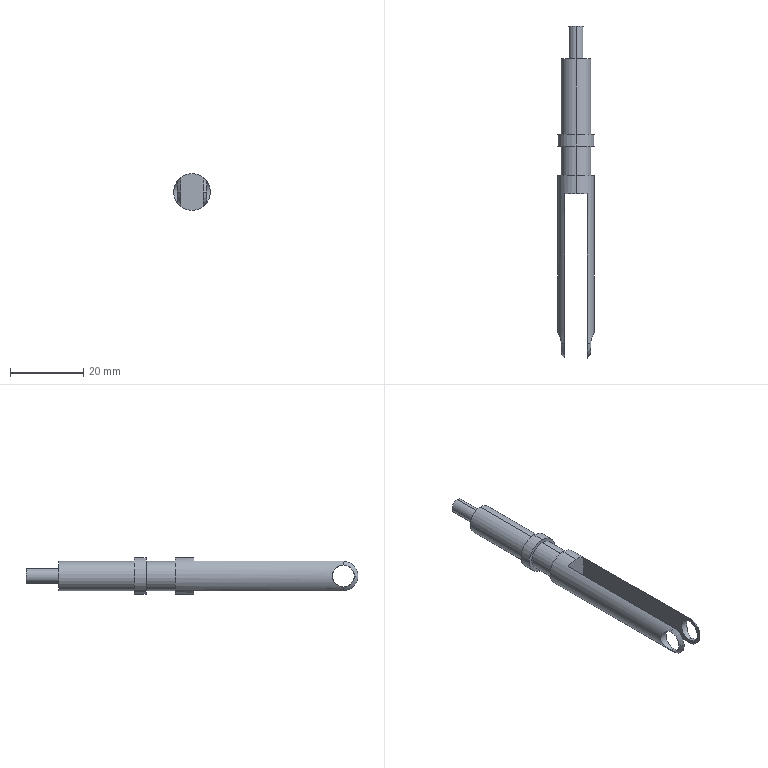Part | SolidWorks | features ICE 2, Revolution 1 | 1 solid | 26 faces | box 10 x 90.414 x 10 mm | volume 3064 mm3 | cylinder 14 | plane 8 | sphere 4 | commonest cylinder face diameters 6 x4 8 x4 10 x4 4 x2
STEP:
#1=CARTESIAN_POINT('',(-29.291,-51.374,3.));
#2=VERTEX_POINT('',#1);
#3=CARTESIAN_POINT('',(-29.291,-51.374,-3.));
#4=VERTEX_POINT('',#3);
#5=CARTESIAN_POINT('',(-29.291,-51.374,0.));
#6=DIRECTION('',(1.,0.,0.));
#7=DIRECTION('',(0.,0.,-1.));
#8=AXIS2_PLACEMENT_3D('',#5,#6,#7);
#9=CIRCLE('',#8,3.);
#10=EDGE_CURVE('',#2,#4,#9,.T.);
#11=ORIENTED_EDGE('',*,*,#10,.F.);
#12=CARTESIAN_POINT('',(-28.291,-51.374,3.));
#13=VERTEX_POINT('',#12);
#14=CARTESIAN_POINT('',(-54.291,-51.374,3.));
#15=DIRECTION('',(1.,0.,0.));
#16=VECTOR('',#15,1000.);
#17=LINE('',#14,#16);
#18=EDGE_CURVE('',#2,#13,#17,.T.);
#19=ORIENTED_EDGE('',*,*,#18,.T.);
#20=CARTESIAN_POINT('',(-28.291,-54.374,0.));
#21=VERTEX_POINT('',#20);
#22=CARTESIAN_POINT('',(-28.291,-51.374,0.));
#23=DIRECTION('',(1.,0.,0.));
#24=DIRECTION('',(0.,0.,1.));
#25=AXIS2_PLACEMENT_3D('',#22,#23,#24);
#26=CIRCLE('',#25,3.);
#27=EDGE_CURVE('',#13,#21,#26,.T.);
#28=ORIENTED_EDGE('',*,*,#27,.T.);
#29=CARTESIAN_POINT('',(-28.291,-51.374,-3.));
#30=VERTEX_POINT('',#29);
#31=CARTESIAN_POINT('',(-28.291,-51.374,0.));
#32=DIRECTION('',(1.,0.,0.));
#33=DIRECTION('',(0.,0.,1.));
#34=AXIS2_PLACEMENT_3D('',#31,#32,#33);
#35=CIRCLE('',#34,3.);
#36=EDGE_CURVE('',#21,#30,#35,.T.);
#37=ORIENTED_EDGE('',*,*,#36,.T.);
#38=CARTESIAN_POINT('',(-54.291,-51.374,-3.));
#39=DIRECTION('',(1.,0.,0.));
#40=VECTOR('',#39,1000.);
#41=LINE('',#38,#40);
#42=EDGE_CURVE('',#4,#30,#41,.T.);
#43=ORIENTED_EDGE('',*,*,#42,.F.);
#44=EDGE_LOOP('',(#11,#19,#28,#37,#43));
#45=FACE_OUTER_BOUND('',#44,.T.);
#46=CARTESIAN_POINT('',(-54.291,-51.374,0.));
#47=DIRECTION('',(1.,0.,0.));
#48=DIRECTION('',(0.,0.,-1.));
#49=AXIS2_PLACEMENT_3D('',#46,#47,#48);
#50=CYLINDRICAL_SURFACE('',#49,3.);
#51=ADVANCED_FACE('',(#45),#50,.F.);
#52=CARTESIAN_POINT('',(-36.291,-54.374,0.));
#53=VERTEX_POINT('',#52);
#54=CARTESIAN_POINT('',(-36.291,-51.374,3.));
#55=VERTEX_POINT('',#54);
#56=CARTESIAN_POINT('',(-36.291,-51.374,0.));
#57=DIRECTION('',(-1.,0.,0.));
#58=DIRECTION('',(0.,0.,-1.));
#59=AXIS2_PLACEMENT_3D('',#56,#57,#58);
#60=CIRCLE('',#59,3.);
#61=EDGE_CURVE('',#53,#55,#60,.T.);
#62=ORIENTED_EDGE('',*,*,#61,.T.);
#63=CARTESIAN_POINT('',(-35.291,-51.374,3.));
#64=VERTEX_POINT('',#63);
#65=CARTESIAN_POINT('',(-54.291,-51.374,3.));
#66=DIRECTION('',(1.,0.,0.));
#67=VECTOR('',#66,1000.);
#68=LINE('',#65,#67);
#69=EDGE_CURVE('',#55,#64,#68,.T.);
#70=ORIENTED_EDGE('',*,*,#69,.T.);
#71=CARTESIAN_POINT('',(-35.291,-51.374,-3.));
#72=VERTEX_POINT('',#71);
#73=CARTESIAN_POINT('',(-35.291,-51.374,0.));
#74=DIRECTION('',(-1.,0.,0.));
#75=DIRECTION('',(0.,0.,1.));
#76=AXIS2_PLACEMENT_3D('',#73,#74,#75);
#77=CIRCLE('',#76,3.);
#78=EDGE_CURVE('',#72,#64,#77,.T.);
#79=ORIENTED_EDGE('',*,*,#78,.F.);
#80=CARTESIAN_POINT('',(-36.291,-51.374,-3.));
#81=VERTEX_POINT('',#80);
#82=CARTESIAN_POINT('',(-54.291,-51.374,-3.));
#83=DIRECTION('',(1.,0.,0.));
#84=VECTOR('',#83,1000.);
#85=LINE('',#82,#84);
#86=EDGE_CURVE('',#81,#72,#85,.T.);
#87=ORIENTED_EDGE('',*,*,#86,.F.);
#88=CARTESIAN_POINT('',(-36.291,-51.374,0.));
#89=DIRECTION('',(-1.,0.,0.));
#90=DIRECTION('',(0.,0.,-1.));
#91=AXIS2_PLACEMENT_3D('',#88,#89,#90);
#92=CIRCLE('',#91,3.);
#93=EDGE_CURVE('',#81,#53,#92,.T.);
#94=ORIENTED_EDGE('',*,*,#93,.T.);
#95=EDGE_LOOP('',(#62,#70,#79,#87,#94));
#96=FACE_OUTER_BOUND('',#95,.T.);
#97=CARTESIAN_POINT('',(-54.291,-51.374,0.));
#98=DIRECTION('',(1.,0.,0.));
#99=DIRECTION('',(0.,0.,-1.));
#100=AXIS2_PLACEMENT_3D('',#97,#98,#99);
#101=CYLINDRICAL_SURFACE('',#100,3.);
#102=ADVANCED_FACE('',(#96),#101,.F.);
#103=ORIENTED_EDGE('',*,*,#61,.F.);
#104=CARTESIAN_POINT('',(-35.291,-55.374,0.));
#105=VERTEX_POINT('',#104);
#106=CARTESIAN_POINT('',(-32.291,-51.374,0.));
#107=DIRECTION('',(0.,0.,1.));
#108=DIRECTION('',(1.,0.,0.));
#109=AXIS2_PLACEMENT_3D('',#106,#107,#108);
#110=CIRCLE('',#109,5.);
#111=EDGE_CURVE('',#53,#105,#110,.T.);
#112=ORIENTED_EDGE('',*,*,#111,.T.);
#113=CARTESIAN_POINT('',(-35.291,-51.374,4.));
#114=VERTEX_POINT('',#113);
#115=CARTESIAN_POINT('',(-35.291,-51.374,0.));
#116=DIRECTION('',(1.,0.,0.));
#117=DIRECTION('',(0.,0.,1.));
#118=AXIS2_PLACEMENT_3D('',#115,#116,#117);
#119=CIRCLE('',#118,4.);
#120=EDGE_CURVE('',#114,#105,#119,.T.);
#121=ORIENTED_EDGE('',*,*,#120,.F.);
#122=CARTESIAN_POINT('',(-32.291,-51.374,0.));
#123=DIRECTION('',(0.,-1.,0.));
#124=DIRECTION('',(0.,0.,-1.));
#125=AXIS2_PLACEMENT_3D('',#122,#123,#124);
#126=CIRCLE('',#125,5.);
#127=EDGE_CURVE('',#114,#55,#126,.T.);
#128=ORIENTED_EDGE('',*,*,#127,.T.);
#129=EDGE_LOOP('',(#103,#112,#121,#128));
#130=FACE_OUTER_BOUND('',#129,.T.);
#131=CARTESIAN_POINT('',(-32.291,-51.374,0.));
#132=DIRECTION('',(0.,0.,-1.));
#133=DIRECTION('',(-1.,0.,0.));
#134=AXIS2_PLACEMENT_3D('',#131,#132,#133);
#135=SPHERICAL_SURFACE('',#134,5.);
#136=ADVANCED_FACE('',(#130),#135,.T.);
#137=CARTESIAN_POINT('',(-32.291,35.041,-2.));
#138=VERTEX_POINT('',#137);
#139=CARTESIAN_POINT('',(-32.291,35.041,2.));
#140=VERTEX_POINT('',#139);
#141=CARTESIAN_POINT('',(-32.291,35.041,0.));
#142=DIRECTION('',(0.,-1.,0.));
#143=DIRECTION('',(0.,0.,-1.));
#144=AXIS2_PLACEMENT_3D('',#141,#142,#143);
#145=CIRCLE('',#144,2.);
#146=EDGE_CURVE('',#138,#140,#145,.T.);
#147=ORIENTED_EDGE('',*,*,#146,.T.);
#148=CARTESIAN_POINT('',(-32.291,26.124,2.));
#149=VERTEX_POINT('',#148);
#150=CARTESIAN_POINT('',(-32.291,35.041,2.));
#151=DIRECTION('',(0.,-1.,0.));
#152=VECTOR('',#151,1000.);
#153=LINE('',#150,#152);
#154=EDGE_CURVE('',#140,#149,#153,.T.);
#155=ORIENTED_EDGE('',*,*,#154,.T.);
#156=CARTESIAN_POINT('',(-32.291,26.124,-2.));
#157=VERTEX_POINT('',#156);
#158=CARTESIAN_POINT('',(-32.291,26.124,0.));
#159=DIRECTION('',(0.,-1.,0.));
#160=DIRECTION('',(0.,0.,-1.));
#161=AXIS2_PLACEMENT_3D('',#158,#159,#160);
#162=CIRCLE('',#161,2.);
#163=EDGE_CURVE('',#157,#149,#162,.T.);
#164=ORIENTED_EDGE('',*,*,#163,.F.);
#165=CARTESIAN_POINT('',(-32.291,35.041,-2.));
#166=DIRECTION('',(0.,-1.,0.));
#167=VECTOR('',#166,1000.);
#168=LINE('',#165,#167);
#169=EDGE_CURVE('',#138,#157,#168,.T.);
#170=ORIENTED_EDGE('',*,*,#169,.F.);
#171=EDGE_LOOP('',(#147,#155,#164,#170));
#172=FACE_OUTER_BOUND('',#171,.T.);
#173=CARTESIAN_POINT('',(-32.291,35.041,0.));
#174=DIRECTION('',(0.,-1.,0.));
#175=DIRECTION('',(0.,0.,-1.));
#176=AXIS2_PLACEMENT_3D('',#173,#174,#175);
#177=CYLINDRICAL_SURFACE('',#176,2.);
#178=ADVANCED_FACE('',(#172),#177,.T.);
#179=CARTESIAN_POINT('',(-32.291,26.124,-4.));
#180=VERTEX_POINT('',#179);
#181=CARTESIAN_POINT('',(-32.291,26.124,4.));
#182=VERTEX_POINT('',#181);
#183=CARTESIAN_POINT('',(-32.291,26.124,0.));
#184=DIRECTION('',(0.,-1.,0.));
#185=DIRECTION('',(0.,0.,-1.));
#186=AXIS2_PLACEMENT_3D('',#183,#184,#185);
#187=CIRCLE('',#186,4.);
#188=EDGE_CURVE('',#180,#182,#187,.T.);
#189=ORIENTED_EDGE('',*,*,#188,.T.);
#190=CARTESIAN_POINT('',(-32.291,5.494,4.));
#191=VERTEX_POINT('',#190);
#192=CARTESIAN_POINT('',(-32.291,35.041,4.));
#193=DIRECTION('',(0.,-1.,0.));
#194=VECTOR('',#193,1000.);
#195=LINE('',#192,#194);
#196=EDGE_CURVE('',#182,#191,#195,.T.);
#197=ORIENTED_EDGE('',*,*,#196,.T.);
#198=CARTESIAN_POINT('',(-32.291,5.494,-4.));
#199=VERTEX_POINT('',#198);
#200=CARTESIAN_POINT('',(-32.291,5.494,0.));
#201=DIRECTION('',(0.,-1.,0.));
#202=DIRECTION('',(0.,0.,-1.));
#203=AXIS2_PLACEMENT_3D('',#200,#201,#202);
#204=CIRCLE('',#203,4.);
#205=EDGE_CURVE('',#199,#191,#204,.T.);
#206=ORIENTED_EDGE('',*,*,#205,.F.);
#207=CARTESIAN_POINT('',(-32.291,35.041,-4.));
#208=DIRECTION('',(0.,-1.,0.));
#209=VECTOR('',#208,1000.);
#210=LINE('',#207,#209);
#211=EDGE_CURVE('',#180,#199,#210,.T.);
#212=ORIENTED_EDGE('',*,*,#211,.F.);
#213=EDGE_LOOP('',(#189,#197,#206,#212));
#214=FACE_OUTER_BOUND('',#213,.T.);
#215=CARTESIAN_POINT('',(-32.291,35.041,0.));
#216=DIRECTION('',(0.,-1.,0.));
#217=DIRECTION('',(0.,0.,-1.));
#218=AXIS2_PLACEMENT_3D('',#215,#216,#217);
#219=CYLINDRICAL_SURFACE('',#218,4.);
#220=ADVANCED_FACE('',(#214),#219,.T.);
#221=CARTESIAN_POINT('',(-32.291,5.494,-5.));
#222=VERTEX_POINT('',#221);
#223=CARTESIAN_POINT('',(-32.291,5.494,5.));
#224=VERTEX_POINT('',#223);
#225=CARTESIAN_POINT('',(-32.291,5.494,0.));
#226=DIRECTION('',(0.,-1.,0.));
#227=DIRECTION('',(0.,0.,-1.));
#228=AXIS2_PLACEMENT_3D('',#225,#226,#227);
#229=CIRCLE('',#228,5.);
#230=EDGE_CURVE('',#222,#224,#229,.T.);
#231=ORIENTED_EDGE('',*,*,#230,.T.);
#232=CARTESIAN_POINT('',(-32.291,2.336,5.));
#233=VERTEX_POINT('',#232);
#234=CARTESIAN_POINT('',(-32.291,35.041,5.));
#235=DIRECTION('',(0.,-1.,0.));
#236=VECTOR('',#235,1000.);
#237=LINE('',#234,#236);
#238=EDGE_CURVE('',#224,#233,#237,.T.);
#239=ORIENTED_EDGE('',*,*,#238,.T.);
#240=CARTESIAN_POINT('',(-32.291,2.336,-5.));
#241=VERTEX_POINT('',#240);
#242=CARTESIAN_POINT('',(-32.291,2.336,0.));
#243=DIRECTION('',(0.,-1.,0.));
#244=DIRECTION('',(0.,0.,-1.));
#245=AXIS2_PLACEMENT_3D('',#242,#243,#244);
#246=CIRCLE('',#245,5.);
#247=EDGE_CURVE('',#241,#233,#246,.T.);
#248=ORIENTED_EDGE('',*,*,#247,.F.);
#249=CARTESIAN_POINT('',(-32.291,35.041,-5.));
#250=DIRECTION('',(0.,-1.,0.));
#251=VECTOR('',#250,1000.);
#252=LINE('',#249,#251);
#253=EDGE_CURVE('',#222,#241,#252,.T.);
#254=ORIENTED_EDGE('',*,*,#253,.F.);
#255=EDGE_LOOP('',(#231,#239,#248,#254));
#256=FACE_OUTER_BOUND('',#255,.T.);
#257=CARTESIAN_POINT('',(-32.291,35.041,0.));
#258=DIRECTION('',(0.,-1.,0.));
#259=DIRECTION('',(0.,0.,-1.));
#260=AXIS2_PLACEMENT_3D('',#257,#258,#259);
#261=CYLINDRICAL_SURFACE('',#260,5.);
#262=ADVANCED_FACE('',(#256),#261,.T.);
#263=CARTESIAN_POINT('',(-32.291,2.336,-4.));
#264=VERTEX_POINT('',#263);
#265=CARTESIAN_POINT('',(-32.291,2.336,4.));
#266=VERTEX_POINT('',#265);
#267=CARTESIAN_POINT('',(-32.291,2.336,0.));
#268=DIRECTION('',(0.,-1.,0.));
#269=DIRECTION('',(0.,0.,-1.));
#270=AXIS2_PLACEMENT_3D('',#267,#268,#269);
#271=CIRCLE('',#270,4.);
#272=EDGE_CURVE('',#264,#266,#271,.T.);
#273=ORIENTED_EDGE('',*,*,#272,.T.);
#274=CARTESIAN_POINT('',(-32.291,-5.664,4.));
#275=VERTEX_POINT('',#274);
#276=CARTESIAN_POINT('',(-32.291,35.041,4.));
#277=DIRECTION('',(0.,-1.,0.));
#278=VECTOR('',#277,1000.);
#279=LINE('',#276,#278);
#280=EDGE_CURVE('',#266,#275,#279,.T.);
#281=ORIENTED_EDGE('',*,*,#280,.T.);
#282=CARTESIAN_POINT('',(-32.291,-5.664,-4.));
#283=VERTEX_POINT('',#282);
#284=CARTESIAN_POINT('',(-32.291,-5.664,0.));
#285=DIRECTION('',(0.,-1.,0.));
#286=DIRECTION('',(0.,0.,-1.));
#287=AXIS2_PLACEMENT_3D('',#284,#285,#286);
#288=CIRCLE('',#287,4.);
#289=EDGE_CURVE('',#283,#275,#288,.T.);
#290=ORIENTED_EDGE('',*,*,#289,.F.);
#291=CARTESIAN_POINT('',(-32.291,35.041,-4.));
#292=DIRECTION('',(0.,-1.,0.));
#293=VECTOR('',#292,1000.);
#294=LINE('',#291,#293);
#295=EDGE_CURVE('',#264,#283,#294,.T.);
#296=ORIENTED_EDGE('',*,*,#295,.F.);
#297=EDGE_LOOP('',(#273,#281,#290,#296));
#298=FACE_OUTER_BOUND('',#297,.T.);
#299=CARTESIAN_POINT('',(-32.291,35.041,0.));
#300=DIRECTION('',(0.,-1.,0.));
#301=DIRECTION('',(0.,0.,-1.));
#302=AXIS2_PLACEMENT_3D('',#299,#300,#301);
#303=CYLINDRICAL_SURFACE('',#302,4.);
#304=ADVANCED_FACE('',(#298),#303,.T.);
#305=CARTESIAN_POINT('',(-32.291,-5.664,-5.));
#306=VERTEX_POINT('',#305);
#307=CARTESIAN_POINT('',(-32.291,-5.664,5.));
#308=VERTEX_POINT('',#307);
#309=CARTESIAN_POINT('',(-32.291,-5.664,0.));
#310=DIRECTION('',(0.,-1.,0.));
#311=DIRECTION('',(0.,0.,-1.));
#312=AXIS2_PLACEMENT_3D('',#309,#310,#311);
#313=CIRCLE('',#312,5.);
#314=EDGE_CURVE('',#306,#308,#313,.T.);
#315=ORIENTED_EDGE('',*,*,#314,.T.);
#316=CARTESIAN_POINT('',(-32.291,-10.664,5.));
#317=VERTEX_POINT('',#316);
#318=CARTESIAN_POINT('',(-32.291,35.041,5.));
#319=DIRECTION('',(0.,-1.,0.));
#320=VECTOR('',#319,1000.);
#321=LINE('',#318,#320);
#322=EDGE_CURVE('',#308,#317,#321,.T.);
#323=ORIENTED_EDGE('',*,*,#322,.T.);
#324=CARTESIAN_POINT('',(-29.291,-10.664,4.));
#325=VERTEX_POINT('',#324);
#326=CARTESIAN_POINT('',(-32.291,-10.664,0.));
#327=DIRECTION('',(0.,1.,0.));
#328=DIRECTION('',(0.,0.,-1.));
#329=AXIS2_PLACEMENT_3D('',#326,#327,#328);
#330=CIRCLE('',#329,5.);
#331=EDGE_CURVE('',#317,#325,#330,.T.);
#332=ORIENTED_EDGE('',*,*,#331,.T.);
#333=CARTESIAN_POINT('',(-29.291,-51.374,4.));
#334=VERTEX_POINT('',#333);
#335=CARTESIAN_POINT('',(-29.291,35.041,4.));
#336=DIRECTION('',(0.,1.,0.));
#337=VECTOR('',#336,1000.);
#338=LINE('',#335,#337);
#339=EDGE_CURVE('',#334,#325,#338,.T.);
#340=ORIENTED_EDGE('',*,*,#339,.F.);
#341=CARTESIAN_POINT('',(-32.291,-51.374,0.));
#342=DIRECTION('',(0.,-1.,0.));
#343=DIRECTION('',(0.,0.,-1.));
#344=AXIS2_PLACEMENT_3D('',#341,#342,#343);
#345=CIRCLE('',#344,5.);
#346=EDGE_CURVE('',#13,#334,#345,.T.);
#347=ORIENTED_EDGE('',*,*,#346,.F.);
#348=CARTESIAN_POINT('',(-28.291,-51.374,-3.));
#349=CARTESIAN_POINT('',(-28.291,-51.17,-3.));
#350=CARTESIAN_POINT('',(-28.275,-50.971,-2.979));
#351=CARTESIAN_POINT('',(-28.218,-50.581,-2.9));
#352=CARTESIAN_POINT('',(-28.175,-50.389,-2.841));
#353=CARTESIAN_POINT('',(-28.025,-49.85,-2.614));
#354=CARTESIAN_POINT('',(-27.892,-49.527,-2.395));
#355=CARTESIAN_POINT('',(-27.702,-49.121,-1.991));
#356=CARTESIAN_POINT('',(-27.639,-48.997,-1.841));
#357=CARTESIAN_POINT('',(-27.525,-48.78,-1.521));
#358=CARTESIAN_POINT('',(-27.474,-48.688,-1.351));
#359=CARTESIAN_POINT('',(-27.387,-48.535,-0.9904));
#360=CARTESIAN_POINT('',(-27.351,-48.474,-0.7969));
#361=CARTESIAN_POINT('',(-27.304,-48.395,-0.4064));
#362=CARTESIAN_POINT('',(-27.291,-48.374,-0.2077));
#363=CARTESIAN_POINT('',(-27.291,-48.373,0.197));
#364=CARTESIAN_POINT('',(-27.303,-48.394,0.3998));
#365=CARTESIAN_POINT('',(-27.35,-48.473,0.7912));
#366=CARTESIAN_POINT('',(-27.385,-48.533,0.9841));
#367=CARTESIAN_POINT('',(-27.516,-48.763,1.529));
#368=CARTESIAN_POINT('',(-27.638,-48.985,1.855));
#369=CARTESIAN_POINT('',(-27.828,-49.391,2.259));
#370=CARTESIAN_POINT('',(-27.893,-49.54,2.382));
#371=CARTESIAN_POINT('',(-28.017,-49.86,2.597));
#372=CARTESIAN_POINT('',(-28.074,-50.028,2.689));
#373=CARTESIAN_POINT('',(-28.175,-50.386,2.84));
#374=CARTESIAN_POINT('',(-28.217,-50.578,2.9));
#375=CARTESIAN_POINT('',(-28.275,-50.97,2.979));
#376=CARTESIAN_POINT('',(-28.291,-51.169,3.));
#377=CARTESIAN_POINT('',(-28.291,-51.374,3.));
#378=B_SPLINE_CURVE_WITH_KNOTS('',3,(#348,#349,#350,#351,#352,#353,#354,#355,#356,#357,#358,#359,#360,#361,#362,#363,#364,#365,#366,#367,#368,#369,#370,#371,#372,#373,#374,#375,#376,#377),.UNSPECIFIED.,.F.,.F.,(4,2,2,2,2,2,2,2,2,2,2,2,2,2,4),(0.,0.0006013,0.001203,0.002405,0.003007,0.003608,0.004209,0.00481,0.005412,0.006013,0.007216,0.007817,0.008418,0.00902,0.009621),.UNSPECIFIED.);
#379=EDGE_CURVE('',#30,#13,#378,.T.);
#380=ORIENTED_EDGE('',*,*,#379,.F.);
#381=CARTESIAN_POINT('',(-29.291,-51.374,-4.));
#382=VERTEX_POINT('',#381);
#383=CARTESIAN_POINT('',(-32.291,-51.374,0.));
#384=DIRECTION('',(0.,-1.,0.));
#385=DIRECTION('',(0.,0.,-1.));
#386=AXIS2_PLACEMENT_3D('',#383,#384,#385);
#387=CIRCLE('',#386,5.);
#388=EDGE_CURVE('',#382,#30,#387,.T.);
#389=ORIENTED_EDGE('',*,*,#388,.F.);
#390=CARTESIAN_POINT('',(-29.291,-10.664,-4.));
#391=VERTEX_POINT('',#390);
#392=CARTESIAN_POINT('',(-29.291,35.041,-4.));
#393=DIRECTION('',(0.,-1.,0.));
#394=VECTOR('',#393,1000.);
#395=LINE('',#392,#394);
#396=EDGE_CURVE('',#391,#382,#395,.T.);
#397=ORIENTED_EDGE('',*,*,#396,.F.);
#398=CARTESIAN_POINT('',(-32.291,-10.664,-5.));
#399=VERTEX_POINT('',#398);
#400=CARTESIAN_POINT('',(-32.291,-10.664,0.));
#401=DIRECTION('',(0.,1.,0.));
#402=DIRECTION('',(0.,0.,-1.));
#403=AXIS2_PLACEMENT_3D('',#400,#401,#402);
#404=CIRCLE('',#403,5.);
#405=EDGE_CURVE('',#391,#399,#404,.T.);
#406=ORIENTED_EDGE('',*,*,#405,.T.);
#407=CARTESIAN_POINT('',(-32.291,35.041,-5.));
#408=DIRECTION('',(0.,-1.,0.));
#409=VECTOR('',#408,1000.);
#410=LINE('',#407,#409);
#411=EDGE_CURVE('',#306,#399,#410,.T.);
#412=ORIENTED_EDGE('',*,*,#411,.F.);
#413=EDGE_LOOP('',(#315,#323,#332,#340,#347,#380,#389,#397,#406,#412));
#414=FACE_OUTER_BOUND('',#413,.T.);
#415=CARTESIAN_POINT('',(-32.291,35.041,0.));
#416=DIRECTION('',(0.,-1.,0.));
#417=DIRECTION('',(0.,0.,-1.));
#418=AXIS2_PLACEMENT_3D('',#415,#416,#417);
#419=CYLINDRICAL_SURFACE('',#418,5.);
#420=ADVANCED_FACE('',(#414),#419,.T.);
#421=ORIENTED_EDGE('',*,*,#36,.F.);
#422=CARTESIAN_POINT('',(-29.291,-55.374,0.));
#423=VERTEX_POINT('',#422);
#424=CARTESIAN_POINT('',(-32.291,-51.374,0.));
#425=DIRECTION('',(0.,0.,-1.));
#426=DIRECTION('',(-1.,0.,0.));
#427=AXIS2_PLACEMENT_3D('',#424,#425,#426);
#428=CIRCLE('',#427,5.);
#429=EDGE_CURVE('',#21,#423,#428,.T.);
#430=ORIENTED_EDGE('',*,*,#429,.T.);
#431=CARTESIAN_POINT('',(-29.291,-51.374,0.));
#432=DIRECTION('',(-1.,0.,0.));
#433=DIRECTION('',(0.,0.,-1.));
#434=AXIS2_PLACEMENT_3D('',#431,#432,#433);
#435=CIRCLE('',#434,4.);
#436=EDGE_CURVE('',#382,#423,#435,.T.);
#437=ORIENTED_EDGE('',*,*,#436,.F.);
#438=ORIENTED_EDGE('',*,*,#388,.T.);
#439=EDGE_LOOP('',(#421,#430,#437,#438));
#440=FACE_OUTER_BOUND('',#439,.T.);
#441=CARTESIAN_POINT('',(-32.291,-51.374,0.));
#442=DIRECTION('',(0.,0.,-1.));
#443=DIRECTION('',(-1.,0.,0.));
#444=AXIS2_PLACEMENT_3D('',#441,#442,#443);
#445=SPHERICAL_SURFACE('',#444,5.);
#446=ADVANCED_FACE('',(#440),#445,.T.);
#447=ORIENTED_EDGE('',*,*,#429,.F.);
#448=ORIENTED_EDGE('',*,*,#27,.F.);
#449=ORIENTED_EDGE('',*,*,#346,.T.);
#450=CARTESIAN_POINT('',(-29.291,-51.374,0.));
#451=DIRECTION('',(-1.,0.,0.));
#452=DIRECTION('',(0.,0.,-1.));
#453=AXIS2_PLACEMENT_3D('',#450,#451,#452);
#454=CIRCLE('',#453,4.);
#455=EDGE_CURVE('',#423,#334,#454,.T.);
#456=ORIENTED_EDGE('',*,*,#455,.F.);
#457=EDGE_LOOP('',(#447,#448,#449,#456));
#458=FACE_OUTER_BOUND('',#457,.T.);
#459=CARTESIAN_POINT('',(-32.291,-51.374,0.));
#460=DIRECTION('',(0.,0.,-1.));
#461=DIRECTION('',(-1.,0.,0.));
#462=AXIS2_PLACEMENT_3D('',#459,#460,#461);
#463=SPHERICAL_SURFACE('',#462,5.);
#464=ADVANCED_FACE('',(#458),#463,.T.);
#465=ORIENTED_EDGE('',*,*,#322,.F.);
#466=CARTESIAN_POINT('',(-32.291,-5.664,0.));
#467=DIRECTION('',(0.,-1.,0.));
#468=DIRECTION('',(0.,0.,-1.));
#469=AXIS2_PLACEMENT_3D('',#466,#467,#468);
#470=CIRCLE('',#469,5.);
#471=EDGE_CURVE('',#308,#306,#470,.T.);
#472=ORIENTED_EDGE('',*,*,#471,.T.);
#473=ORIENTED_EDGE('',*,*,#411,.T.);
#474=CARTESIAN_POINT('',(-35.291,-10.664,-4.));
#475=VERTEX_POINT('',#474);
#476=CARTESIAN_POINT('',(-32.291,-10.664,0.));
#477=DIRECTION('',(0.,1.,0.));
#478=DIRECTION('',(0.,0.,-1.));
#479=AXIS2_PLACEMENT_3D('',#476,#477,#478);
#480=CIRCLE('',#479,5.);
#481=EDGE_CURVE('',#399,#475,#480,.T.);
#482=ORIENTED_EDGE('',*,*,#481,.T.);
#483=CARTESIAN_POINT('',(-35.291,-51.374,-4.));
#484=VERTEX_POINT('',#483);
#485=CARTESIAN_POINT('',(-35.291,35.041,-4.));
#486=DIRECTION('',(0.,1.,0.));
#487=VECTOR('',#486,1000.);
#488=LINE('',#485,#487);
#489=EDGE_CURVE('',#484,#475,#488,.T.);
#490=ORIENTED_EDGE('',*,*,#489,.F.);
#491=CARTESIAN_POINT('',(-32.291,-51.374,0.));
#492=DIRECTION('',(0.,-1.,0.));
#493=DIRECTION('',(0.,0.,-1.));
#494=AXIS2_PLACEMENT_3D('',#491,#492,#493);
#495=CIRCLE('',#494,5.);
#496=EDGE_CURVE('',#81,#484,#495,.T.);
#497=ORIENTED_EDGE('',*,*,#496,.F.);
#498=CARTESIAN_POINT('',(-36.291,-51.374,3.));
#499=CARTESIAN_POINT('',(-36.291,-51.17,3.));
#500=CARTESIAN_POINT('',(-36.307,-50.971,2.979));
#501=CARTESIAN_POINT('',(-36.364,-50.581,2.9));
#502=CARTESIAN_POINT('',(-36.407,-50.389,2.841));
#503=CARTESIAN_POINT('',(-36.558,-49.85,2.614));
#504=CARTESIAN_POINT('',(-36.69,-49.527,2.395));
#505=CARTESIAN_POINT('',(-36.88,-49.121,1.991));
#506=CARTESIAN_POINT('',(-36.943,-48.997,1.841));
#507=CARTESIAN_POINT('',(-37.057,-48.78,1.521));
#508=CARTESIAN_POINT('',(-37.109,-48.688,1.351));
#509=CARTESIAN_POINT('',(-37.196,-48.535,0.9904));
#510=CARTESIAN_POINT('',(-37.231,-48.474,0.7969));
#511=CARTESIAN_POINT('',(-37.278,-48.395,0.4064));
#512=CARTESIAN_POINT('',(-37.291,-48.374,0.2077));
#513=CARTESIAN_POINT('',(-37.291,-48.373,-0.197));
#514=CARTESIAN_POINT('',(-37.279,-48.394,-0.3998));
#515=CARTESIAN_POINT('',(-37.232,-48.473,-0.7912));
#516=CARTESIAN_POINT('',(-37.197,-48.533,-0.9841));
#517=CARTESIAN_POINT('',(-37.066,-48.763,-1.529));
#518=CARTESIAN_POINT('',(-36.944,-48.985,-1.855));
#519=CARTESIAN_POINT('',(-36.754,-49.391,-2.259));
#520=CARTESIAN_POINT('',(-36.689,-49.54,-2.382));
#521=CARTESIAN_POINT('',(-36.566,-49.86,-2.597));
#522=CARTESIAN_POINT('',(-36.508,-50.028,-2.689));
#523=CARTESIAN_POINT('',(-36.408,-50.386,-2.84));
#524=CARTESIAN_POINT('',(-36.365,-50.578,-2.9));
#525=CARTESIAN_POINT('',(-36.307,-50.97,-2.979));
#526=CARTESIAN_POINT('',(-36.291,-51.169,-3.));
#527=CARTESIAN_POINT('',(-36.291,-51.374,-3.));
#528=B_SPLINE_CURVE_WITH_KNOTS('',3,(#498,#499,#500,#501,#502,#503,#504,#505,#506,#507,#508,#509,#510,#511,#512,#513,#514,#515,#516,#517,#518,#519,#520,#521,#522,#523,#524,#525,#526,#527),.UNSPECIFIED.,.F.,.F.,(4,2,2,2,2,2,2,2,2,2,2,2,2,2,4),(0.,0.0006013,0.001203,0.002405,0.003007,0.003608,0.004209,0.00481,0.005412,0.006013,0.007216,0.007817,0.008418,0.00902,0.009621),.UNSPECIFIED.);
#529=EDGE_CURVE('',#55,#81,#528,.T.);
#530=ORIENTED_EDGE('',*,*,#529,.F.);
#531=ORIENTED_EDGE('',*,*,#127,.F.);
#532=CARTESIAN_POINT('',(-35.291,-10.664,4.));
#533=VERTEX_POINT('',#532);
#534=CARTESIAN_POINT('',(-35.291,35.041,4.));
#535=DIRECTION('',(0.,-1.,0.));
#536=VECTOR('',#535,1000.);
#537=LINE('',#534,#536);
#538=EDGE_CURVE('',#533,#114,#537,.T.);
#539=ORIENTED_EDGE('',*,*,#538,.F.);
#540=CARTESIAN_POINT('',(-32.291,-10.664,0.));
#541=DIRECTION('',(0.,1.,0.));
#542=DIRECTION('',(0.,0.,-1.));
#543=AXIS2_PLACEMENT_3D('',#540,#541,#542);
#544=CIRCLE('',#543,5.);
#545=EDGE_CURVE('',#533,#317,#544,.T.);
#546=ORIENTED_EDGE('',*,*,#545,.T.);
#547=EDGE_LOOP('',(#465,#472,#473,#482,#490,#497,#530,#531,#539,#546));
#548=FACE_OUTER_BOUND('',#547,.T.);
#549=CARTESIAN_POINT('',(-32.291,35.041,0.));
#550=DIRECTION('',(0.,-1.,0.));
#551=DIRECTION('',(0.,0.,-1.));
#552=AXIS2_PLACEMENT_3D('',#549,#550,#551);
#553=CYLINDRICAL_SURFACE('',#552,5.);
#554=ADVANCED_FACE('',(#548),#553,.T.);
#555=ORIENTED_EDGE('',*,*,#289,.T.);
#556=CARTESIAN_POINT('',(-32.291,-5.664,0.));
#557=DIRECTION('',(0.,-1.,0.));
#558=DIRECTION('',(0.,0.,-1.));
#559=AXIS2_PLACEMENT_3D('',#556,#557,#558);
#560=CIRCLE('',#559,4.);
#561=EDGE_CURVE('',#275,#283,#560,.T.);
#562=ORIENTED_EDGE('',*,*,#561,.T.);
#563=EDGE_LOOP('',(#555,#562));
#564=FACE_BOUND('',#563,.T.);
#565=ORIENTED_EDGE('',*,*,#314,.F.);
#566=ORIENTED_EDGE('',*,*,#471,.F.);
#567=EDGE_LOOP('',(#565,#566));
#568=FACE_OUTER_BOUND('',#567,.T.);
#569=CARTESIAN_POINT('',(-27.291,-5.664,0.));
#570=DIRECTION('',(0.,1.,0.));
#571=DIRECTION('',(0.,0.,1.));
#572=AXIS2_PLACEMENT_3D('',#569,#570,#571);
#573=PLANE('',#572);
#574=ADVANCED_FACE('',(#564,#568),#573,.T.);
#575=ORIENTED_EDGE('',*,*,#280,.F.);
#576=CARTESIAN_POINT('',(-32.291,2.336,0.));
#577=DIRECTION('',(0.,-1.,0.));
#578=DIRECTION('',(0.,0.,-1.));
#579=AXIS2_PLACEMENT_3D('',#576,#577,#578);
#580=CIRCLE('',#579,4.);
#581=EDGE_CURVE('',#266,#264,#580,.T.);
#582=ORIENTED_EDGE('',*,*,#581,.T.);
#583=ORIENTED_EDGE('',*,*,#295,.T.);
#584=ORIENTED_EDGE('',*,*,#561,.F.);
#585=EDGE_LOOP('',(#575,#582,#583,#584));
#586=FACE_OUTER_BOUND('',#585,.T.);
#587=CARTESIAN_POINT('',(-32.291,35.041,0.));
#588=DIRECTION('',(0.,-1.,0.));
#589=DIRECTION('',(0.,0.,-1.));
#590=AXIS2_PLACEMENT_3D('',#587,#588,#589);
#591=CYLINDRICAL_SURFACE('',#590,4.);
#592=ADVANCED_FACE('',(#586),#591,.T.);
#593=ORIENTED_EDGE('',*,*,#247,.T.);
#594=CARTESIAN_POINT('',(-32.291,2.336,0.));
#595=DIRECTION('',(0.,-1.,0.));
#596=DIRECTION('',(0.,0.,-1.));
#597=AXIS2_PLACEMENT_3D('',#594,#595,#596);
#598=CIRCLE('',#597,5.);
#599=EDGE_CURVE('',#233,#241,#598,.T.);
#600=ORIENTED_EDGE('',*,*,#599,.T.);
#601=EDGE_LOOP('',(#593,#600));
#602=FACE_OUTER_BOUND('',#601,.T.);
#603=ORIENTED_EDGE('',*,*,#272,.F.);
#604=ORIENTED_EDGE('',*,*,#581,.F.);
#605=EDGE_LOOP('',(#603,#604));
#606=FACE_BOUND('',#605,.T.);
#607=CARTESIAN_POINT('',(-28.291,2.336,0.));
#608=DIRECTION('',(0.,-1.,0.));
#609=DIRECTION('',(0.,0.,-1.));
#610=AXIS2_PLACEMENT_3D('',#607,#608,#609);
#611=PLANE('',#610);
#612=ADVANCED_FACE('',(#602,#606),#611,.T.);
#613=ORIENTED_EDGE('',*,*,#238,.F.);
#614=CARTESIAN_POINT('',(-32.291,5.494,0.));
#615=DIRECTION('',(0.,-1.,0.));
#616=DIRECTION('',(0.,0.,-1.));
#617=AXIS2_PLACEMENT_3D('',#614,#615,#616);
#618=CIRCLE('',#617,5.);
#619=EDGE_CURVE('',#224,#222,#618,.T.);
#620=ORIENTED_EDGE('',*,*,#619,.T.);
#621=ORIENTED_EDGE('',*,*,#253,.T.);
#622=ORIENTED_EDGE('',*,*,#599,.F.);
#623=EDGE_LOOP('',(#613,#620,#621,#622));
#624=FACE_OUTER_BOUND('',#623,.T.);
#625=CARTESIAN_POINT('',(-32.291,35.041,0.));
#626=DIRECTION('',(0.,-1.,0.));
#627=DIRECTION('',(0.,0.,-1.));
#628=AXIS2_PLACEMENT_3D('',#625,#626,#627);
#629=CYLINDRICAL_SURFACE('',#628,5.);
#630=ADVANCED_FACE('',(#624),#629,.T.);
#631=ORIENTED_EDGE('',*,*,#205,.T.);
#632=CARTESIAN_POINT('',(-32.291,5.494,0.));
#633=DIRECTION('',(0.,-1.,0.));
#634=DIRECTION('',(0.,0.,-1.));
#635=AXIS2_PLACEMENT_3D('',#632,#633,#634);
#636=CIRCLE('',#635,4.);
#637=EDGE_CURVE('',#191,#199,#636,.T.);
#638=ORIENTED_EDGE('',*,*,#637,.T.);
#639=EDGE_LOOP('',(#631,#638));
#640=FACE_BOUND('',#639,.T.);
#641=ORIENTED_EDGE('',*,*,#230,.F.);
#642=ORIENTED_EDGE('',*,*,#619,.F.);
#643=EDGE_LOOP('',(#641,#642));
#644=FACE_OUTER_BOUND('',#643,.T.);
#645=CARTESIAN_POINT('',(-27.291,5.494,0.));
#646=DIRECTION('',(0.,1.,0.));
#647=DIRECTION('',(0.,0.,1.));
#648=AXIS2_PLACEMENT_3D('',#645,#646,#647);
#649=PLANE('',#648);
#650=ADVANCED_FACE('',(#640,#644),#649,.T.);
#651=ORIENTED_EDGE('',*,*,#196,.F.);
#652=CARTESIAN_POINT('',(-32.291,26.124,0.));
#653=DIRECTION('',(0.,-1.,0.));
#654=DIRECTION('',(0.,0.,-1.));
#655=AXIS2_PLACEMENT_3D('',#652,#653,#654);
#656=CIRCLE('',#655,4.);
#657=EDGE_CURVE('',#182,#180,#656,.T.);
#658=ORIENTED_EDGE('',*,*,#657,.T.);
#659=ORIENTED_EDGE('',*,*,#211,.T.);
#660=ORIENTED_EDGE('',*,*,#637,.F.);
#661=EDGE_LOOP('',(#651,#658,#659,#660));
#662=FACE_OUTER_BOUND('',#661,.T.);
#663=CARTESIAN_POINT('',(-32.291,35.041,0.));
#664=DIRECTION('',(0.,-1.,0.));
#665=DIRECTION('',(0.,0.,-1.));
#666=AXIS2_PLACEMENT_3D('',#663,#664,#665);
#667=CYLINDRICAL_SURFACE('',#666,4.);
#668=ADVANCED_FACE('',(#662),#667,.T.);
#669=ORIENTED_EDGE('',*,*,#163,.T.);
#670=CARTESIAN_POINT('',(-32.291,26.124,0.));
#671=DIRECTION('',(0.,-1.,0.));
#672=DIRECTION('',(0.,0.,-1.));
#673=AXIS2_PLACEMENT_3D('',#670,#671,#672);
#674=CIRCLE('',#673,2.);
#675=EDGE_CURVE('',#149,#157,#674,.T.);
#676=ORIENTED_EDGE('',*,*,#675,.T.);
#677=EDGE_LOOP('',(#669,#676));
#678=FACE_BOUND('',#677,.T.);
#679=ORIENTED_EDGE('',*,*,#188,.F.);
#680=ORIENTED_EDGE('',*,*,#657,.F.);
#681=EDGE_LOOP('',(#679,#680));
#682=FACE_OUTER_BOUND('',#681,.T.);
#683=CARTESIAN_POINT('',(-28.291,26.124,0.));
#684=DIRECTION('',(0.,1.,0.));
#685=DIRECTION('',(0.,0.,1.));
#686=AXIS2_PLACEMENT_3D('',#683,#684,#685);
#687=PLANE('',#686);
#688=ADVANCED_FACE('',(#678,#682),#687,.T.);
#689=ORIENTED_EDGE('',*,*,#154,.F.);
#690=CARTESIAN_POINT('',(-32.291,35.041,0.));
#691=DIRECTION('',(0.,-1.,0.));
#692=DIRECTION('',(0.,0.,-1.));
#693=AXIS2_PLACEMENT_3D('',#690,#691,#692);
#694=CIRCLE('',#693,2.);
#695=EDGE_CURVE('',#140,#138,#694,.T.);
#696=ORIENTED_EDGE('',*,*,#695,.T.);
#697=ORIENTED_EDGE('',*,*,#169,.T.);
#698=ORIENTED_EDGE('',*,*,#675,.F.);
#699=EDGE_LOOP('',(#689,#696,#697,#698));
#700=FACE_OUTER_BOUND('',#699,.T.);
#701=CARTESIAN_POINT('',(-32.291,35.041,0.));
#702=DIRECTION('',(0.,-1.,0.));
#703=DIRECTION('',(0.,0.,-1.));
#704=AXIS2_PLACEMENT_3D('',#701,#702,#703);
#705=CYLINDRICAL_SURFACE('',#704,2.);
#706=ADVANCED_FACE('',(#700),#705,.T.);
#707=ORIENTED_EDGE('',*,*,#146,.F.);
#708=ORIENTED_EDGE('',*,*,#695,.F.);
#709=EDGE_LOOP('',(#707,#708));
#710=FACE_OUTER_BOUND('',#709,.T.);
#711=CARTESIAN_POINT('',(-32.291,35.041,0.));
#712=DIRECTION('',(0.,1.,0.));
#713=DIRECTION('',(0.,0.,1.));
#714=AXIS2_PLACEMENT_3D('',#711,#712,#713);
#715=PLANE('',#714);
#716=ADVANCED_FACE('',(#710),#715,.T.);
#717=ORIENTED_EDGE('',*,*,#111,.F.);
#718=ORIENTED_EDGE('',*,*,#93,.F.);
#719=ORIENTED_EDGE('',*,*,#496,.T.);
#720=CARTESIAN_POINT('',(-35.291,-51.374,0.));
#721=DIRECTION('',(1.,0.,0.));
#722=DIRECTION('',(0.,0.,1.));
#723=AXIS2_PLACEMENT_3D('',#720,#721,#722);
#724=CIRCLE('',#723,4.);
#725=EDGE_CURVE('',#105,#484,#724,.T.);
#726=ORIENTED_EDGE('',*,*,#725,.F.);
#727=EDGE_LOOP('',(#717,#718,#719,#726));
#728=FACE_OUTER_BOUND('',#727,.T.);
#729=CARTESIAN_POINT('',(-32.291,-51.374,0.));
#730=DIRECTION('',(0.,0.,-1.));
#731=DIRECTION('',(-1.,0.,0.));
#732=AXIS2_PLACEMENT_3D('',#729,#730,#731);
#733=SPHERICAL_SURFACE('',#732,5.);
#734=ADVANCED_FACE('',(#728),#733,.T.);
#735=CARTESIAN_POINT('',(-29.291,-51.374,0.));
#736=DIRECTION('',(1.,0.,0.));
#737=DIRECTION('',(0.,0.,-1.));
#738=AXIS2_PLACEMENT_3D('',#735,#736,#737);
#739=CIRCLE('',#738,3.);
#740=EDGE_CURVE('',#4,#2,#739,.T.);
#741=ORIENTED_EDGE('',*,*,#740,.T.);
#742=ORIENTED_EDGE('',*,*,#10,.T.);
#743=EDGE_LOOP('',(#741,#742));
#744=FACE_BOUND('',#743,.T.);
#745=ORIENTED_EDGE('',*,*,#339,.T.);
#746=CARTESIAN_POINT('',(-29.291,-10.664,-9.117));
#747=DIRECTION('',(0.,0.,1.));
#748=VECTOR('',#747,1000.);
#749=LINE('',#746,#748);
#750=EDGE_CURVE('',#391,#325,#749,.T.);
#751=ORIENTED_EDGE('',*,*,#750,.F.);
#752=ORIENTED_EDGE('',*,*,#396,.T.);
#753=ORIENTED_EDGE('',*,*,#436,.T.);
#754=ORIENTED_EDGE('',*,*,#455,.T.);
#755=EDGE_LOOP('',(#745,#751,#752,#753,#754));
#756=FACE_OUTER_BOUND('',#755,.T.);
#757=CARTESIAN_POINT('',(-29.291,-10.664,-9.117));
#758=DIRECTION('',(1.,0.,0.));
#759=DIRECTION('',(0.,0.,-1.));
#760=AXIS2_PLACEMENT_3D('',#757,#758,#759);
#761=PLANE('',#760);
#762=ADVANCED_FACE('',(#744,#756),#761,.F.);
#763=ORIENTED_EDGE('',*,*,#78,.T.);
#764=CARTESIAN_POINT('',(-35.291,-51.374,0.));
#765=DIRECTION('',(-1.,0.,0.));
#766=DIRECTION('',(0.,0.,1.));
#767=AXIS2_PLACEMENT_3D('',#764,#765,#766);
#768=CIRCLE('',#767,3.);
#769=EDGE_CURVE('',#64,#72,#768,.T.);
#770=ORIENTED_EDGE('',*,*,#769,.T.);
#771=EDGE_LOOP('',(#763,#770));
#772=FACE_BOUND('',#771,.T.);
#773=ORIENTED_EDGE('',*,*,#489,.T.);
#774=CARTESIAN_POINT('',(-35.291,-10.664,-9.117));
#775=DIRECTION('',(0.,0.,-1.));
#776=VECTOR('',#775,1000.);
#777=LINE('',#774,#776);
#778=EDGE_CURVE('',#533,#475,#777,.T.);
#779=ORIENTED_EDGE('',*,*,#778,.F.);
#780=ORIENTED_EDGE('',*,*,#538,.T.);
#781=ORIENTED_EDGE('',*,*,#120,.T.);
#782=ORIENTED_EDGE('',*,*,#725,.T.);
#783=EDGE_LOOP('',(#773,#779,#780,#781,#782));
#784=FACE_OUTER_BOUND('',#783,.T.);
#785=CARTESIAN_POINT('',(-35.291,-10.664,-9.117));
#786=DIRECTION('',(-1.,0.,0.));
#787=DIRECTION('',(0.,0.,1.));
#788=AXIS2_PLACEMENT_3D('',#785,#786,#787);
#789=PLANE('',#788);
#790=ADVANCED_FACE('',(#772,#784),#789,.F.);
#791=ORIENTED_EDGE('',*,*,#778,.T.);
#792=ORIENTED_EDGE('',*,*,#481,.F.);
#793=ORIENTED_EDGE('',*,*,#405,.F.);
#794=ORIENTED_EDGE('',*,*,#750,.T.);
#795=ORIENTED_EDGE('',*,*,#331,.F.);
#796=ORIENTED_EDGE('',*,*,#545,.F.);
#797=EDGE_LOOP('',(#791,#792,#793,#794,#795,#796));
#798=FACE_OUTER_BOUND('',#797,.T.);
#799=CARTESIAN_POINT('',(0.,-10.664,0.));
#800=DIRECTION('',(0.,-1.,0.));
#801=DIRECTION('',(0.,0.,-1.));
#802=AXIS2_PLACEMENT_3D('',#799,#800,#801);
#803=PLANE('',#802);
#804=ADVANCED_FACE('',(#798),#803,.T.);
#805=ORIENTED_EDGE('',*,*,#69,.F.);
#806=ORIENTED_EDGE('',*,*,#529,.T.);
#807=ORIENTED_EDGE('',*,*,#86,.T.);
#808=ORIENTED_EDGE('',*,*,#769,.F.);
#809=EDGE_LOOP('',(#805,#806,#807,#808));
#810=FACE_OUTER_BOUND('',#809,.T.);
#811=CARTESIAN_POINT('',(-54.291,-51.374,0.));
#812=DIRECTION('',(1.,0.,0.));
#813=DIRECTION('',(0.,0.,-1.));
#814=AXIS2_PLACEMENT_3D('',#811,#812,#813);
#815=CYLINDRICAL_SURFACE('',#814,3.);
#816=ADVANCED_FACE('',(#810),#815,.F.);
#817=ORIENTED_EDGE('',*,*,#18,.F.);
#818=ORIENTED_EDGE('',*,*,#740,.F.);
#819=ORIENTED_EDGE('',*,*,#42,.T.);
#820=ORIENTED_EDGE('',*,*,#379,.T.);
#821=EDGE_LOOP('',(#817,#818,#819,#820));
#822=FACE_OUTER_BOUND('',#821,.T.);
#823=CARTESIAN_POINT('',(-54.291,-51.374,0.));
#824=DIRECTION('',(1.,0.,0.));
#825=DIRECTION('',(0.,0.,-1.));
#826=AXIS2_PLACEMENT_3D('',#823,#824,#825);
#827=CYLINDRICAL_SURFACE('',#826,3.);
#828=ADVANCED_FACE('',(#822),#827,.F.);
#829=CLOSED_SHELL('',(#51,#102,#136,#178,#220,#262,#304,#420,#446,#464,#554,#574,#592,#612,#630,#650,#668,#688,#706,#716,#734,#762,#790,#804,#816,#828));
#830=MANIFOLD_SOLID_BREP('',#829);
#831=CARTESIAN_POINT('',(0.,0.,0.));
#832=DIRECTION('',(0.,0.,1.));
#833=DIRECTION('',(1.,0.,0.));
#834=AXIS2_PLACEMENT_3D('',#831,#832,#833);
#835=(LENGTH_UNIT()NAMED_UNIT(*)SI_UNIT(.MILLI.,.METRE.));
#836=UNCERTAINTY_MEASURE_WITH_UNIT(LENGTH_MEASURE(0.00001),#835,'','');
#837=(NAMED_UNIT(*)PLANE_ANGLE_UNIT()SI_UNIT($,.RADIAN.));
#838=(NAMED_UNIT(*)SI_UNIT($,.STERADIAN.)SOLID_ANGLE_UNIT());
#839=(GEOMETRIC_REPRESENTATION_CONTEXT(3)GLOBAL_UNCERTAINTY_ASSIGNED_CONTEXT((#836))GLOBAL_UNIT_ASSIGNED_CONTEXT((#835,#837,#838))REPRESENTATION_CONTEXT('',''));
#840=ADVANCED_BREP_SHAPE_REPRESENTATION('',(#830,#834),#839);